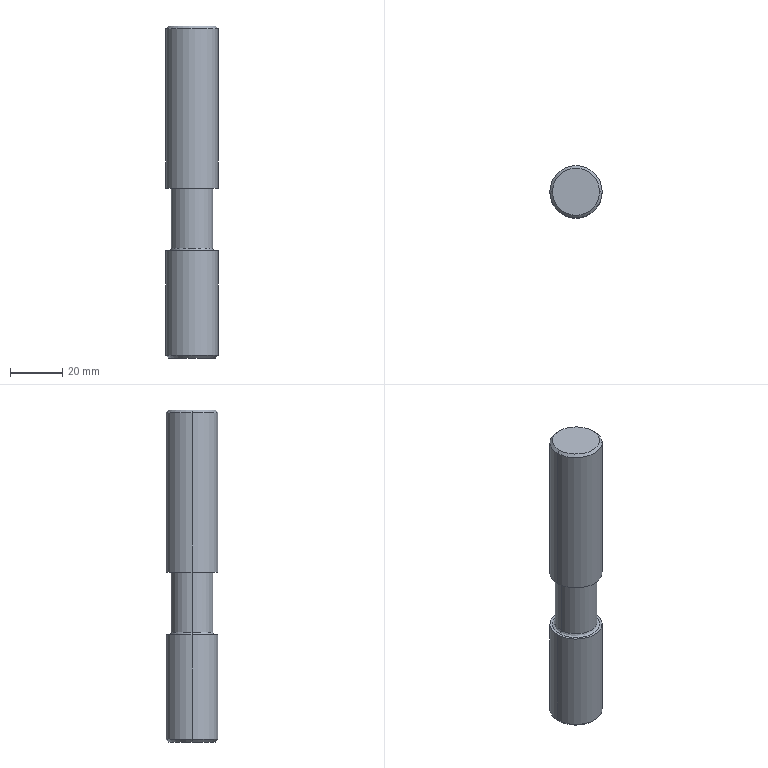Part | STEP file | 1 solid | 16 faces | box 20 x 20 x 127 mm | volume 37133 mm3 | cylinder 6 | plane 4 | cone 4 | spline 2 | commonest cylinder face diameters 20 x4 16 x2